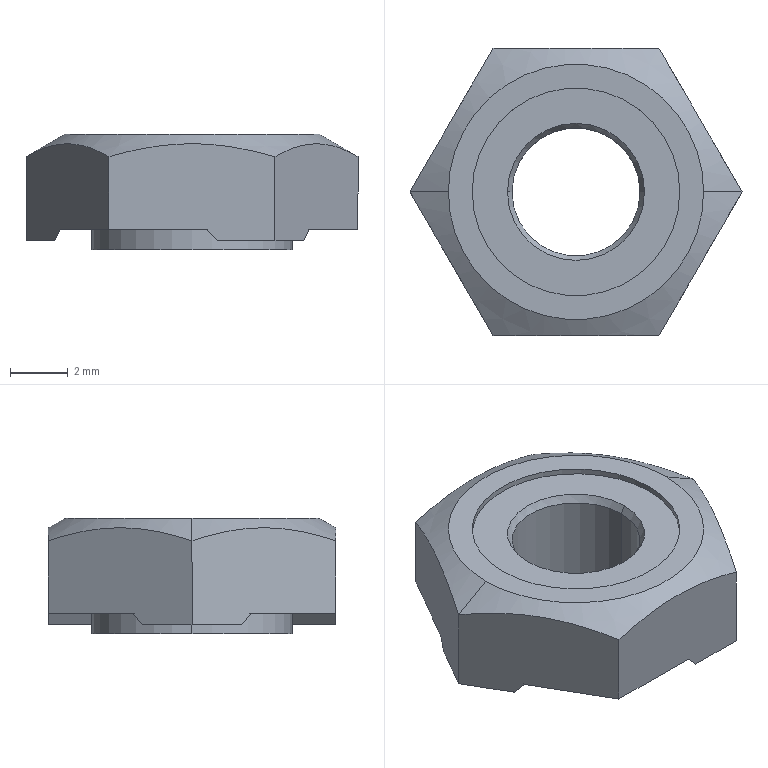Part | SolidWorks | features Cut 2, RevCut 2, Boss 1, Chamfer 1, CirPattern 1, Draft 1, Extrusion 1, LPattern 1, RefAxis 1 | 1 solid | 28 faces | box 11.547 x 10 x 4 mm | volume 240.353 mm3 | plane 16 | cone 6 | cylinder 6 | commonest cylinder face diameters 4.459 x2 6.96 x2 7.22 x2
STEP:
#1=CARTESIAN_POINT('',(-2.229,0.,-0.4667));
#2=VERTEX_POINT('',#1);
#3=CARTESIAN_POINT('',(2.229,0.,-0.4667));
#4=VERTEX_POINT('',#3);
#5=CARTESIAN_POINT('',(0.,0.,-0.4667));
#6=DIRECTION('',(0.,0.,1.));
#7=DIRECTION('',(-1.,0.,0.));
#8=AXIS2_PLACEMENT_3D('',#5,#6,#7);
#9=CIRCLE('',#8,2.229);
#10=EDGE_CURVE('',#2,#4,#9,.T.);
#11=ORIENTED_EDGE('',*,*,#10,.F.);
#12=CARTESIAN_POINT('',(-2.383,0.,-0.2));
#13=VERTEX_POINT('',#12);
#14=CARTESIAN_POINT('',(-2.383,0.,-0.2));
#15=DIRECTION('',(-0.5,0.,0.866));
#16=VECTOR('',#15,1000.);
#17=LINE('',#14,#16);
#18=EDGE_CURVE('',#2,#13,#17,.T.);
#19=ORIENTED_EDGE('',*,*,#18,.T.);
#20=CARTESIAN_POINT('',(2.383,0.,-0.2));
#21=VERTEX_POINT('',#20);
#22=CARTESIAN_POINT('',(0.,0.,-0.2));
#23=DIRECTION('',(0.,0.,-1.));
#24=DIRECTION('',(-1.,0.,0.));
#25=AXIS2_PLACEMENT_3D('',#22,#23,#24);
#26=CIRCLE('',#25,2.383);
#27=EDGE_CURVE('',#21,#13,#26,.T.);
#28=ORIENTED_EDGE('',*,*,#27,.F.);
#29=CARTESIAN_POINT('',(2.383,0.,-0.2));
#30=DIRECTION('',(0.5,0.,0.866));
#31=VECTOR('',#30,1000.);
#32=LINE('',#29,#31);
#33=EDGE_CURVE('',#4,#21,#32,.T.);
#34=ORIENTED_EDGE('',*,*,#33,.F.);
#35=EDGE_LOOP('',(#11,#19,#28,#34));
#36=FACE_OUTER_BOUND('',#35,.T.);
#37=CARTESIAN_POINT('',(0.,0.,-0.2));
#38=DIRECTION('',(0.,0.,1.));
#39=DIRECTION('',(1.,0.,0.));
#40=AXIS2_PLACEMENT_3D('',#37,#38,#39);
#41=CONICAL_SURFACE('',#40,2.383,0.5236);
#42=ADVANCED_FACE('',(#36),#41,.F.);
#43=CARTESIAN_POINT('',(2.229,0.,-3.846));
#44=VERTEX_POINT('',#43);
#45=CARTESIAN_POINT('',(-2.229,0.,-3.846));
#46=VERTEX_POINT('',#45);
#47=CARTESIAN_POINT('',(0.,0.,-3.846));
#48=DIRECTION('',(0.,0.,-1.));
#49=DIRECTION('',(1.,0.,0.));
#50=AXIS2_PLACEMENT_3D('',#47,#48,#49);
#51=CIRCLE('',#50,2.229);
#52=EDGE_CURVE('',#44,#46,#51,.T.);
#53=ORIENTED_EDGE('',*,*,#52,.F.);
#54=CARTESIAN_POINT('',(2.496,0.,-4.));
#55=VERTEX_POINT('',#54);
#56=CARTESIAN_POINT('',(2.229,0.,-3.846));
#57=DIRECTION('',(0.866,0.,-0.5));
#58=VECTOR('',#57,1000.);
#59=LINE('',#56,#58);
#60=EDGE_CURVE('',#44,#55,#59,.T.);
#61=ORIENTED_EDGE('',*,*,#60,.T.);
#62=CARTESIAN_POINT('',(-2.496,0.,-4.));
#63=VERTEX_POINT('',#62);
#64=CARTESIAN_POINT('',(0.,0.,-4.));
#65=DIRECTION('',(0.,0.,1.));
#66=DIRECTION('',(1.,0.,0.));
#67=AXIS2_PLACEMENT_3D('',#64,#65,#66);
#68=CIRCLE('',#67,2.496);
#69=EDGE_CURVE('',#63,#55,#68,.T.);
#70=ORIENTED_EDGE('',*,*,#69,.F.);
#71=CARTESIAN_POINT('',(-2.229,0.,-3.846));
#72=DIRECTION('',(-0.866,0.,-0.5));
#73=VECTOR('',#72,1000.);
#74=LINE('',#71,#73);
#75=EDGE_CURVE('',#46,#63,#74,.T.);
#76=ORIENTED_EDGE('',*,*,#75,.F.);
#77=EDGE_LOOP('',(#53,#61,#70,#76));
#78=FACE_OUTER_BOUND('',#77,.T.);
#79=CARTESIAN_POINT('',(0.,0.,-3.846));
#80=DIRECTION('',(0.,0.,-1.));
#81=DIRECTION('',(-1.,0.,0.));
#82=AXIS2_PLACEMENT_3D('',#79,#80,#81);
#83=CONICAL_SURFACE('',#82,2.229,1.047);
#84=ADVANCED_FACE('',(#78),#83,.F.);
#85=ORIENTED_EDGE('',*,*,#10,.T.);
#86=CARTESIAN_POINT('',(2.229,0.,0.));
#87=DIRECTION('',(0.,0.,-1.));
#88=VECTOR('',#87,1000.);
#89=LINE('',#86,#88);
#90=EDGE_CURVE('',#4,#44,#89,.T.);
#91=ORIENTED_EDGE('',*,*,#90,.T.);
#92=ORIENTED_EDGE('',*,*,#52,.T.);
#93=CARTESIAN_POINT('',(-2.229,0.,0.));
#94=DIRECTION('',(0.,0.,-1.));
#95=VECTOR('',#94,1000.);
#96=LINE('',#93,#95);
#97=EDGE_CURVE('',#2,#46,#96,.T.);
#98=ORIENTED_EDGE('',*,*,#97,.F.);
#99=EDGE_LOOP('',(#85,#91,#92,#98));
#100=FACE_OUTER_BOUND('',#99,.T.);
#101=CARTESIAN_POINT('',(0.,0.,0.));
#102=DIRECTION('',(0.,0.,-1.));
#103=DIRECTION('',(-1.,0.,0.));
#104=AXIS2_PLACEMENT_3D('',#101,#102,#103);
#105=CYLINDRICAL_SURFACE('',#104,2.229);
#106=ADVANCED_FACE('',(#100),#105,.F.);
#107=CARTESIAN_POINT('',(-3.48,0.,-3.3));
#108=VERTEX_POINT('',#107);
#109=CARTESIAN_POINT('',(3.48,0.,-3.3));
#110=VERTEX_POINT('',#109);
#111=CARTESIAN_POINT('',(0.,0.,-3.3));
#112=DIRECTION('',(0.,0.,-1.));
#113=DIRECTION('',(-1.,0.,0.));
#114=AXIS2_PLACEMENT_3D('',#111,#112,#113);
#115=CIRCLE('',#114,3.48);
#116=EDGE_CURVE('',#108,#110,#115,.T.);
#117=ORIENTED_EDGE('',*,*,#116,.T.);
#118=CARTESIAN_POINT('',(3.48,0.,-4.));
#119=VERTEX_POINT('',#118);
#120=CARTESIAN_POINT('',(3.48,0.,-3.3));
#121=DIRECTION('',(0.,0.,-1.));
#122=VECTOR('',#121,1000.);
#123=LINE('',#120,#122);
#124=EDGE_CURVE('',#110,#119,#123,.T.);
#125=ORIENTED_EDGE('',*,*,#124,.T.);
#126=CARTESIAN_POINT('',(-3.48,0.,-4.));
#127=VERTEX_POINT('',#126);
#128=CARTESIAN_POINT('',(0.,0.,-4.));
#129=DIRECTION('',(0.,0.,-1.));
#130=DIRECTION('',(-1.,0.,0.));
#131=AXIS2_PLACEMENT_3D('',#128,#129,#130);
#132=CIRCLE('',#131,3.48);
#133=EDGE_CURVE('',#127,#119,#132,.T.);
#134=ORIENTED_EDGE('',*,*,#133,.F.);
#135=CARTESIAN_POINT('',(-3.48,0.,-3.3));
#136=DIRECTION('',(0.,0.,-1.));
#137=VECTOR('',#136,1000.);
#138=LINE('',#135,#137);
#139=EDGE_CURVE('',#108,#127,#138,.T.);
#140=ORIENTED_EDGE('',*,*,#139,.F.);
#141=EDGE_LOOP('',(#117,#125,#134,#140));
#142=FACE_OUTER_BOUND('',#141,.T.);
#143=CARTESIAN_POINT('',(0.,0.,-3.3));
#144=DIRECTION('',(0.,0.,-1.));
#145=DIRECTION('',(-1.,0.,0.));
#146=AXIS2_PLACEMENT_3D('',#143,#144,#145);
#147=CYLINDRICAL_SURFACE('',#146,3.48);
#148=ADVANCED_FACE('',(#142),#147,.T.);
#149=CARTESIAN_POINT('',(3.61,0.,0.));
#150=VERTEX_POINT('',#149);
#151=CARTESIAN_POINT('',(-3.61,0.,0.));
#152=VERTEX_POINT('',#151);
#153=CARTESIAN_POINT('',(0.,0.,0.));
#154=DIRECTION('',(0.,0.,-1.));
#155=DIRECTION('',(-1.,0.,0.));
#156=AXIS2_PLACEMENT_3D('',#153,#154,#155);
#157=CIRCLE('',#156,3.61);
#158=EDGE_CURVE('',#150,#152,#157,.T.);
#159=ORIENTED_EDGE('',*,*,#158,.F.);
#160=CARTESIAN_POINT('',(3.61,0.,-0.2));
#161=VERTEX_POINT('',#160);
#162=CARTESIAN_POINT('',(3.61,0.,-9.902));
#163=DIRECTION('',(0.,0.,-1.));
#164=VECTOR('',#163,1000.);
#165=LINE('',#162,#164);
#166=EDGE_CURVE('',#150,#161,#165,.T.);
#167=ORIENTED_EDGE('',*,*,#166,.T.);
#168=CARTESIAN_POINT('',(-3.61,0.,-0.2));
#169=VERTEX_POINT('',#168);
#170=CARTESIAN_POINT('',(0.,0.,-0.2));
#171=DIRECTION('',(0.,0.,-1.));
#172=DIRECTION('',(-1.,0.,0.));
#173=AXIS2_PLACEMENT_3D('',#170,#171,#172);
#174=CIRCLE('',#173,3.61);
#175=EDGE_CURVE('',#161,#169,#174,.T.);
#176=ORIENTED_EDGE('',*,*,#175,.T.);
#177=CARTESIAN_POINT('',(-3.61,0.,-9.902));
#178=DIRECTION('',(0.,0.,-1.));
#179=VECTOR('',#178,1000.);
#180=LINE('',#177,#179);
#181=EDGE_CURVE('',#152,#169,#180,.T.);
#182=ORIENTED_EDGE('',*,*,#181,.F.);
#183=EDGE_LOOP('',(#159,#167,#176,#182));
#184=FACE_OUTER_BOUND('',#183,.T.);
#185=CARTESIAN_POINT('',(0.,0.,-9.902));
#186=DIRECTION('',(0.,0.,-1.));
#187=DIRECTION('',(-1.,0.,0.));
#188=AXIS2_PLACEMENT_3D('',#185,#186,#187);
#189=CYLINDRICAL_SURFACE('',#188,3.61);
#190=ADVANCED_FACE('',(#184),#189,.F.);
#191=CARTESIAN_POINT('',(-4.44,0.,0.));
#192=VERTEX_POINT('',#191);
#193=CARTESIAN_POINT('',(4.44,0.,0.));
#194=VERTEX_POINT('',#193);
#195=CARTESIAN_POINT('',(0.,0.,0.));
#196=DIRECTION('',(0.,0.,-1.));
#197=DIRECTION('',(-1.,0.,0.));
#198=AXIS2_PLACEMENT_3D('',#195,#196,#197);
#199=CIRCLE('',#198,4.44);
#200=EDGE_CURVE('',#192,#194,#199,.T.);
#201=ORIENTED_EDGE('',*,*,#200,.T.);
#202=CARTESIAN_POINT('',(5.774,0.,-0.7699));
#203=VERTEX_POINT('',#202);
#204=CARTESIAN_POINT('',(4.44,0.,0.));
#205=DIRECTION('',(0.866,0.,-0.5));
#206=VECTOR('',#205,1000.);
#207=LINE('',#204,#206);
#208=EDGE_CURVE('',#194,#203,#207,.T.);
#209=ORIENTED_EDGE('',*,*,#208,.T.);
#210=CARTESIAN_POINT('',(2.887,5.,-0.7699));
#211=VERTEX_POINT('',#210);
#212=CARTESIAN_POINT('',(5.774,0.,-0.7699));
#213=CARTESIAN_POINT('',(5.302,0.8164,-0.4978));
#214=CARTESIAN_POINT('',(4.824,1.645,-0.3239));
#215=CARTESIAN_POINT('',(4.21,2.708,-0.3232));
#216=CARTESIAN_POINT('',(4.087,2.921,-0.3336));
#217=CARTESIAN_POINT('',(3.843,3.344,-0.3743));
#218=CARTESIAN_POINT('',(3.722,3.554,-0.4045));
#219=CARTESIAN_POINT('',(3.361,4.179,-0.5212));
#220=CARTESIAN_POINT('',(3.123,4.591,-0.6337));
#221=CARTESIAN_POINT('',(2.887,5.,-0.7699));
#222=B_SPLINE_CURVE_WITH_KNOTS('',3,(#212,#213,#214,#215,#216,#217,#218,#219,#220,#221),.UNSPECIFIED.,.F.,.F.,(4,2,2,2,4),(0.000000238,0.002916,0.003645,0.004373,0.005831),.UNSPECIFIED.);
#223=EDGE_CURVE('',#203,#211,#222,.T.);
#224=ORIENTED_EDGE('',*,*,#223,.T.);
#225=CARTESIAN_POINT('',(-2.887,5.,-0.7699));
#226=VERTEX_POINT('',#225);
#227=CARTESIAN_POINT('',(2.887,5.,-0.7699));
#228=CARTESIAN_POINT('',(2.42,5.,-0.6352));
#229=CARTESIAN_POINT('',(1.947,5.,-0.523));
#230=CARTESIAN_POINT('',(0.9831,5.,-0.3664));
#231=CARTESIAN_POINT('',(0.4886,5.,-0.3234));
#232=CARTESIAN_POINT('',(-0.487,5.,-0.3233));
#233=CARTESIAN_POINT('',(-0.9718,5.,-0.3652));
#234=CARTESIAN_POINT('',(-1.936,5.,-0.5206));
#235=CARTESIAN_POINT('',(-2.417,5.,-0.6344));
#236=CARTESIAN_POINT('',(-2.887,5.,-0.7699));
#237=B_SPLINE_CURVE_WITH_KNOTS('',3,(#227,#228,#229,#230,#231,#232,#233,#234,#235,#236),.UNSPECIFIED.,.F.,.F.,(4,2,2,2,4),(0.01286,0.01432,0.01578,0.01724,0.01871),.UNSPECIFIED.);
#238=EDGE_CURVE('',#211,#226,#237,.T.);
#239=ORIENTED_EDGE('',*,*,#238,.T.);
#240=CARTESIAN_POINT('',(-5.774,0.,-0.7699));
#241=VERTEX_POINT('',#240);
#242=CARTESIAN_POINT('',(-2.887,5.,-0.7699));
#243=CARTESIAN_POINT('',(-3.358,4.184,-0.4978));
#244=CARTESIAN_POINT('',(-3.837,3.355,-0.3239));
#245=CARTESIAN_POINT('',(-4.45,2.292,-0.3232));
#246=CARTESIAN_POINT('',(-4.573,2.079,-0.3336));
#247=CARTESIAN_POINT('',(-4.817,1.656,-0.3743));
#248=CARTESIAN_POINT('',(-4.938,1.446,-0.4045));
#249=CARTESIAN_POINT('',(-5.3,0.8208,-0.5212));
#250=CARTESIAN_POINT('',(-5.538,0.4087,-0.6337));
#251=CARTESIAN_POINT('',(-5.774,0.,-0.7699));
#252=B_SPLINE_CURVE_WITH_KNOTS('',3,(#242,#243,#244,#245,#246,#247,#248,#249,#250,#251),.UNSPECIFIED.,.F.,.F.,(4,2,2,2,4),(0.000000238,0.002916,0.003645,0.004373,0.005831),.UNSPECIFIED.);
#253=EDGE_CURVE('',#226,#241,#252,.T.);
#254=ORIENTED_EDGE('',*,*,#253,.T.);
#255=CARTESIAN_POINT('',(-4.44,0.,0.));
#256=DIRECTION('',(-0.866,0.,-0.5));
#257=VECTOR('',#256,1000.);
#258=LINE('',#255,#257);
#259=EDGE_CURVE('',#192,#241,#258,.T.);
#260=ORIENTED_EDGE('',*,*,#259,.F.);
#261=EDGE_LOOP('',(#201,#209,#224,#239,#254,#260));
#262=FACE_OUTER_BOUND('',#261,.T.);
#263=CARTESIAN_POINT('',(0.,0.,0.));
#264=DIRECTION('',(0.,0.,-1.));
#265=DIRECTION('',(-1.,0.,0.));
#266=AXIS2_PLACEMENT_3D('',#263,#264,#265);
#267=CONICAL_SURFACE('',#266,4.44,1.047);
#268=ADVANCED_FACE('',(#262),#267,.T.);
#269=ORIENTED_EDGE('',*,*,#116,.F.);
#270=CARTESIAN_POINT('',(0.,0.,-3.3));
#271=DIRECTION('',(0.,0.,-1.));
#272=DIRECTION('',(-1.,0.,0.));
#273=AXIS2_PLACEMENT_3D('',#270,#271,#272);
#274=CIRCLE('',#273,3.48);
#275=EDGE_CURVE('',#110,#108,#274,.T.);
#276=ORIENTED_EDGE('',*,*,#275,.F.);
#277=EDGE_LOOP('',(#269,#276));
#278=FACE_BOUND('',#277,.T.);
#279=CARTESIAN_POINT('',(-4.587,-2.055,-3.3));
#280=VERTEX_POINT('',#279);
#281=CARTESIAN_POINT('',(-2.887,-5.,-3.3));
#282=VERTEX_POINT('',#281);
#283=CARTESIAN_POINT('',(-5.774,0.,-3.3));
#284=DIRECTION('',(0.5,-0.866,0.));
#285=VECTOR('',#284,1000.);
#286=LINE('',#283,#285);
#287=EDGE_CURVE('',#280,#282,#286,.T.);
#288=ORIENTED_EDGE('',*,*,#287,.F.);
#289=CARTESIAN_POINT('',(-4.587,2.055,-3.3));
#290=VERTEX_POINT('',#289);
#291=CARTESIAN_POINT('',(-4.587,1.732,-3.3));
#292=DIRECTION('',(0.,-1.,0.));
#293=VECTOR('',#292,1000.);
#294=LINE('',#291,#293);
#295=EDGE_CURVE('',#290,#280,#294,.T.);
#296=ORIENTED_EDGE('',*,*,#295,.F.);
#297=CARTESIAN_POINT('',(-2.887,5.,-3.3));
#298=VERTEX_POINT('',#297);
#299=CARTESIAN_POINT('',(-2.887,5.,-3.3));
#300=DIRECTION('',(-0.5,-0.866,0.));
#301=VECTOR('',#300,1000.);
#302=LINE('',#299,#301);
#303=EDGE_CURVE('',#298,#290,#302,.T.);
#304=ORIENTED_EDGE('',*,*,#303,.F.);
#305=CARTESIAN_POINT('',(0.5137,5.,-3.3));
#306=VERTEX_POINT('',#305);
#307=CARTESIAN_POINT('',(2.887,5.,-3.3));
#308=DIRECTION('',(-1.,0.,0.));
#309=VECTOR('',#308,1000.);
#310=LINE('',#307,#309);
#311=EDGE_CURVE('',#306,#298,#310,.T.);
#312=ORIENTED_EDGE('',*,*,#311,.F.);
#313=CARTESIAN_POINT('',(4.073,2.945,-3.3));
#314=VERTEX_POINT('',#313);
#315=CARTESIAN_POINT('',(3.793,3.106,-3.3));
#316=DIRECTION('',(-0.866,0.5,0.));
#317=VECTOR('',#316,1000.);
#318=LINE('',#315,#317);
#319=EDGE_CURVE('',#314,#306,#318,.T.);
#320=ORIENTED_EDGE('',*,*,#319,.F.);
#321=CARTESIAN_POINT('',(5.774,0.,-3.3));
#322=VERTEX_POINT('',#321);
#323=CARTESIAN_POINT('',(5.774,0.,-3.3));
#324=DIRECTION('',(-0.5,0.866,0.));
#325=VECTOR('',#324,1000.);
#326=LINE('',#323,#325);
#327=EDGE_CURVE('',#322,#314,#326,.T.);
#328=ORIENTED_EDGE('',*,*,#327,.F.);
#329=CARTESIAN_POINT('',(4.073,-2.945,-3.3));
#330=VERTEX_POINT('',#329);
#331=CARTESIAN_POINT('',(2.887,-5.,-3.3));
#332=DIRECTION('',(0.5,0.866,0.));
#333=VECTOR('',#332,1000.);
#334=LINE('',#331,#333);
#335=EDGE_CURVE('',#330,#322,#334,.T.);
#336=ORIENTED_EDGE('',*,*,#335,.F.);
#337=CARTESIAN_POINT('',(0.5137,-5.,-3.3));
#338=VERTEX_POINT('',#337);
#339=CARTESIAN_POINT('',(0.7935,-4.838,-3.3));
#340=DIRECTION('',(0.866,0.5,0.));
#341=VECTOR('',#340,1000.);
#342=LINE('',#339,#341);
#343=EDGE_CURVE('',#338,#330,#342,.T.);
#344=ORIENTED_EDGE('',*,*,#343,.F.);
#345=CARTESIAN_POINT('',(-2.887,-5.,-3.3));
#346=DIRECTION('',(1.,0.,0.));
#347=VECTOR('',#346,1000.);
#348=LINE('',#345,#347);
#349=EDGE_CURVE('',#282,#338,#348,.T.);
#350=ORIENTED_EDGE('',*,*,#349,.F.);
#351=EDGE_LOOP('',(#288,#296,#304,#312,#320,#328,#336,#344,#350));
#352=FACE_OUTER_BOUND('',#351,.T.);
#353=CARTESIAN_POINT('',(0.,0.,-3.3));
#354=DIRECTION('',(0.,0.,-1.));
#355=DIRECTION('',(-1.,0.,0.));
#356=AXIS2_PLACEMENT_3D('',#353,#354,#355);
#357=PLANE('',#356);
#358=ADVANCED_FACE('',(#278,#352),#357,.T.);
#359=CARTESIAN_POINT('',(-2.887,-5.,-0.7699));
#360=VERTEX_POINT('',#359);
#361=CARTESIAN_POINT('',(-2.887,-5.,-4.));
#362=DIRECTION('',(0.,0.,1.));
#363=VECTOR('',#362,1000.);
#364=LINE('',#361,#363);
#365=EDGE_CURVE('',#282,#360,#364,.T.);
#366=ORIENTED_EDGE('',*,*,#365,.F.);
#367=ORIENTED_EDGE('',*,*,#349,.T.);
#368=CARTESIAN_POINT('',(0.8868,-5.,-3.7));
#369=VERTEX_POINT('',#368);
#370=CARTESIAN_POINT('',(-0.719,-5.,-1.978));
#371=DIRECTION('',(-0.682,0.,0.7313));
#372=VECTOR('',#371,1000.);
#373=LINE('',#370,#372);
#374=EDGE_CURVE('',#369,#338,#373,.T.);
#375=ORIENTED_EDGE('',*,*,#374,.F.);
#376=CARTESIAN_POINT('',(2.887,-5.,-3.7));
#377=VERTEX_POINT('',#376);
#378=CARTESIAN_POINT('',(2.887,-5.,-3.7));
#379=DIRECTION('',(-1.,0.,0.));
#380=VECTOR('',#379,1000.);
#381=LINE('',#378,#380);
#382=EDGE_CURVE('',#377,#369,#381,.T.);
#383=ORIENTED_EDGE('',*,*,#382,.F.);
#384=CARTESIAN_POINT('',(2.887,-5.,-0.7699));
#385=VERTEX_POINT('',#384);
#386=CARTESIAN_POINT('',(2.887,-5.,-4.));
#387=DIRECTION('',(0.,0.,1.));
#388=VECTOR('',#387,1000.);
#389=LINE('',#386,#388);
#390=EDGE_CURVE('',#377,#385,#389,.T.);
#391=ORIENTED_EDGE('',*,*,#390,.T.);
#392=CARTESIAN_POINT('',(-2.887,-5.,-0.7699));
#393=CARTESIAN_POINT('',(-2.417,-5.,-0.6344));
#394=CARTESIAN_POINT('',(-1.936,-5.,-0.5206));
#395=CARTESIAN_POINT('',(-0.9718,-5.,-0.3652));
#396=CARTESIAN_POINT('',(-0.487,-5.,-0.3233));
#397=CARTESIAN_POINT('',(0.4886,-5.,-0.3234));
#398=CARTESIAN_POINT('',(0.9831,-5.,-0.3664));
#399=CARTESIAN_POINT('',(1.947,-5.,-0.523));
#400=CARTESIAN_POINT('',(2.42,-5.,-0.6352));
#401=CARTESIAN_POINT('',(2.887,-5.,-0.7699));
#402=B_SPLINE_CURVE_WITH_KNOTS('',3,(#392,#393,#394,#395,#396,#397,#398,#399,#400,#401),.UNSPECIFIED.,.F.,.F.,(4,2,2,2,4),(0.005101,0.006561,0.008021,0.009482,0.01094),.UNSPECIFIED.);
#403=EDGE_CURVE('',#360,#385,#402,.T.);
#404=ORIENTED_EDGE('',*,*,#403,.F.);
#405=EDGE_LOOP('',(#366,#367,#375,#383,#391,#404));
#406=FACE_OUTER_BOUND('',#405,.T.);
#407=CARTESIAN_POINT('',(-2.887,-5.,-4.));
#408=DIRECTION('',(0.,-1.,0.));
#409=DIRECTION('',(0.,0.,-1.));
#410=AXIS2_PLACEMENT_3D('',#407,#408,#409);
#411=PLANE('',#410);
#412=ADVANCED_FACE('',(#406),#411,.T.);
#413=CARTESIAN_POINT('',(-5.774,0.,-3.7));
#414=VERTEX_POINT('',#413);
#415=CARTESIAN_POINT('',(-5.774,0.,-4.));
#416=DIRECTION('',(0.,0.,1.));
#417=VECTOR('',#416,1000.);
#418=LINE('',#415,#417);
#419=EDGE_CURVE('',#414,#241,#418,.T.);
#420=ORIENTED_EDGE('',*,*,#419,.F.);
#421=CARTESIAN_POINT('',(-4.774,-1.732,-3.7));
#422=VERTEX_POINT('',#421);
#423=CARTESIAN_POINT('',(-4.774,-1.732,-3.7));
#424=DIRECTION('',(-0.5,0.866,0.));
#425=VECTOR('',#424,1000.);
#426=LINE('',#423,#425);
#427=EDGE_CURVE('',#422,#414,#426,.T.);
#428=ORIENTED_EDGE('',*,*,#427,.F.);
#429=CARTESIAN_POINT('',(-5.471,-0.5235,-5.196));
#430=DIRECTION('',(0.341,-0.5907,0.7313));
#431=VECTOR('',#430,1000.);
#432=LINE('',#429,#431);
#433=EDGE_CURVE('',#422,#280,#432,.T.);
#434=ORIENTED_EDGE('',*,*,#433,.T.);
#435=ORIENTED_EDGE('',*,*,#287,.T.);
#436=ORIENTED_EDGE('',*,*,#365,.T.);
#437=CARTESIAN_POINT('',(-5.774,0.,-0.7699));
#438=CARTESIAN_POINT('',(-5.302,-0.8164,-0.4978));
#439=CARTESIAN_POINT('',(-4.824,-1.645,-0.3239));
#440=CARTESIAN_POINT('',(-4.21,-2.708,-0.3232));
#441=CARTESIAN_POINT('',(-4.087,-2.921,-0.3336));
#442=CARTESIAN_POINT('',(-3.843,-3.344,-0.3743));
#443=CARTESIAN_POINT('',(-3.722,-3.554,-0.4045));
#444=CARTESIAN_POINT('',(-3.361,-4.179,-0.5212));
#445=CARTESIAN_POINT('',(-3.123,-4.591,-0.6337));
#446=CARTESIAN_POINT('',(-2.887,-5.,-0.7699));
#447=B_SPLINE_CURVE_WITH_KNOTS('',3,(#437,#438,#439,#440,#441,#442,#443,#444,#445,#446),.UNSPECIFIED.,.F.,.F.,(4,2,2,2,4),(0.000000238,0.002916,0.003645,0.004373,0.005831),.UNSPECIFIED.);
#448=EDGE_CURVE('',#241,#360,#447,.T.);
#449=ORIENTED_EDGE('',*,*,#448,.F.);
#450=EDGE_LOOP('',(#420,#428,#434,#435,#436,#449));
#451=FACE_OUTER_BOUND('',#450,.T.);
#452=CARTESIAN_POINT('',(-5.774,0.,-4.));
#453=DIRECTION('',(-0.866,-0.5,0.));
#454=DIRECTION('',(0.5,-0.866,0.));
#455=AXIS2_PLACEMENT_3D('',#452,#453,#454);
#456=PLANE('',#455);
#457=ADVANCED_FACE('',(#451),#456,.T.);
#458=CARTESIAN_POINT('',(-2.887,5.,-4.));
#459=DIRECTION('',(0.,0.,1.));
#460=VECTOR('',#459,1000.);
#461=LINE('',#458,#460);
#462=EDGE_CURVE('',#298,#226,#461,.T.);
#463=ORIENTED_EDGE('',*,*,#462,.F.);
#464=ORIENTED_EDGE('',*,*,#303,.T.);
#465=CARTESIAN_POINT('',(-4.774,1.732,-3.7));
#466=VERTEX_POINT('',#465);
#467=CARTESIAN_POINT('',(-3.971,3.123,-1.978));
#468=DIRECTION('',(0.341,0.5907,0.7313));
#469=VECTOR('',#468,1000.);
#470=LINE('',#467,#469);
#471=EDGE_CURVE('',#466,#290,#470,.T.);
#472=ORIENTED_EDGE('',*,*,#471,.F.);
#473=CARTESIAN_POINT('',(-5.774,0.,-3.7));
#474=DIRECTION('',(0.5,0.866,0.));
#475=VECTOR('',#474,1000.);
#476=LINE('',#473,#475);
#477=EDGE_CURVE('',#414,#466,#476,.T.);
#478=ORIENTED_EDGE('',*,*,#477,.F.);
#479=ORIENTED_EDGE('',*,*,#419,.T.);
#480=ORIENTED_EDGE('',*,*,#253,.F.);
#481=EDGE_LOOP('',(#463,#464,#472,#478,#479,#480));
#482=FACE_OUTER_BOUND('',#481,.T.);
#483=CARTESIAN_POINT('',(-2.887,5.,-4.));
#484=DIRECTION('',(-0.866,0.5,0.));
#485=DIRECTION('',(-0.5,-0.866,0.));
#486=AXIS2_PLACEMENT_3D('',#483,#484,#485);
#487=PLANE('',#486);
#488=ADVANCED_FACE('',(#482),#487,.T.);
#489=CARTESIAN_POINT('',(2.887,5.,-3.7));
#490=VERTEX_POINT('',#489);
#491=CARTESIAN_POINT('',(2.887,5.,-4.));
#492=DIRECTION('',(0.,0.,1.));
#493=VECTOR('',#492,1000.);
#494=LINE('',#491,#493);
#495=EDGE_CURVE('',#490,#211,#494,.T.);
#496=ORIENTED_EDGE('',*,*,#495,.F.);
#497=CARTESIAN_POINT('',(0.8868,5.,-3.7));
#498=VERTEX_POINT('',#497);
#499=CARTESIAN_POINT('',(0.8868,5.,-3.7));
#500=DIRECTION('',(1.,0.,0.));
#501=VECTOR('',#500,1000.);
#502=LINE('',#499,#501);
#503=EDGE_CURVE('',#498,#490,#502,.T.);
#504=ORIENTED_EDGE('',*,*,#503,.F.);
#505=CARTESIAN_POINT('',(2.282,5.,-5.196));
#506=DIRECTION('',(-0.682,0.,0.7313));
#507=VECTOR('',#506,1000.);
#508=LINE('',#505,#507);
#509=EDGE_CURVE('',#498,#306,#508,.T.);
#510=ORIENTED_EDGE('',*,*,#509,.T.);
#511=ORIENTED_EDGE('',*,*,#311,.T.);
#512=ORIENTED_EDGE('',*,*,#462,.T.);
#513=ORIENTED_EDGE('',*,*,#238,.F.);
#514=EDGE_LOOP('',(#496,#504,#510,#511,#512,#513));
#515=FACE_OUTER_BOUND('',#514,.T.);
#516=CARTESIAN_POINT('',(2.887,5.,-4.));
#517=DIRECTION('',(0.,1.,0.));
#518=DIRECTION('',(0.,0.,1.));
#519=AXIS2_PLACEMENT_3D('',#516,#517,#518);
#520=PLANE('',#519);
#521=ADVANCED_FACE('',(#515),#520,.T.);
#522=CARTESIAN_POINT('',(5.774,0.,-4.));
#523=DIRECTION('',(0.,0.,1.));
#524=VECTOR('',#523,1000.);
#525=LINE('',#522,#524);
#526=EDGE_CURVE('',#322,#203,#525,.T.);
#527=ORIENTED_EDGE('',*,*,#526,.F.);
#528=ORIENTED_EDGE('',*,*,#327,.T.);
#529=CARTESIAN_POINT('',(3.887,3.268,-3.7));
#530=VERTEX_POINT('',#529);
#531=CARTESIAN_POINT('',(4.69,1.877,-1.978));
#532=DIRECTION('',(0.341,-0.5907,0.7313));
#533=VECTOR('',#532,1000.);
#534=LINE('',#531,#533);
#535=EDGE_CURVE('',#530,#314,#534,.T.);
#536=ORIENTED_EDGE('',*,*,#535,.F.);
#537=CARTESIAN_POINT('',(2.887,5.,-3.7));
#538=DIRECTION('',(0.5,-0.866,0.));
#539=VECTOR('',#538,1000.);
#540=LINE('',#537,#539);
#541=EDGE_CURVE('',#490,#530,#540,.T.);
#542=ORIENTED_EDGE('',*,*,#541,.F.);
#543=ORIENTED_EDGE('',*,*,#495,.T.);
#544=ORIENTED_EDGE('',*,*,#223,.F.);
#545=EDGE_LOOP('',(#527,#528,#536,#542,#543,#544));
#546=FACE_OUTER_BOUND('',#545,.T.);
#547=CARTESIAN_POINT('',(5.774,0.,-4.));
#548=DIRECTION('',(0.866,0.5,0.));
#549=DIRECTION('',(-0.5,0.866,0.));
#550=AXIS2_PLACEMENT_3D('',#547,#548,#549);
#551=PLANE('',#550);
#552=ADVANCED_FACE('',(#546),#551,.T.);
#553=ORIENTED_EDGE('',*,*,#390,.F.);
#554=CARTESIAN_POINT('',(3.887,-3.268,-3.7));
#555=VERTEX_POINT('',#554);
#556=CARTESIAN_POINT('',(3.887,-3.268,-3.7));
#557=DIRECTION('',(-0.5,-0.866,0.));
#558=VECTOR('',#557,1000.);
#559=LINE('',#556,#558);
#560=EDGE_CURVE('',#555,#377,#559,.T.);
#561=ORIENTED_EDGE('',*,*,#560,.F.);
#562=CARTESIAN_POINT('',(3.189,-4.477,-5.196));
#563=DIRECTION('',(0.341,0.5907,0.7313));
#564=VECTOR('',#563,1000.);
#565=LINE('',#562,#564);
#566=EDGE_CURVE('',#555,#330,#565,.T.);
#567=ORIENTED_EDGE('',*,*,#566,.T.);
#568=ORIENTED_EDGE('',*,*,#335,.T.);
#569=ORIENTED_EDGE('',*,*,#526,.T.);
#570=CARTESIAN_POINT('',(2.887,-5.,-0.7699));
#571=CARTESIAN_POINT('',(3.358,-4.184,-0.4978));
#572=CARTESIAN_POINT('',(3.837,-3.355,-0.3239));
#573=CARTESIAN_POINT('',(4.45,-2.292,-0.3232));
#574=CARTESIAN_POINT('',(4.573,-2.079,-0.3336));
#575=CARTESIAN_POINT('',(4.817,-1.656,-0.3743));
#576=CARTESIAN_POINT('',(4.938,-1.446,-0.4045));
#577=CARTESIAN_POINT('',(5.3,-0.8208,-0.5212));
#578=CARTESIAN_POINT('',(5.538,-0.4087,-0.6337));
#579=CARTESIAN_POINT('',(5.774,0.,-0.7699));
#580=B_SPLINE_CURVE_WITH_KNOTS('',3,(#570,#571,#572,#573,#574,#575,#576,#577,#578,#579),.UNSPECIFIED.,.F.,.F.,(4,2,2,2,4),(0.000000238,0.002916,0.003645,0.004373,0.005831),.UNSPECIFIED.);
#581=EDGE_CURVE('',#385,#203,#580,.T.);
#582=ORIENTED_EDGE('',*,*,#581,.F.);
#583=EDGE_LOOP('',(#553,#561,#567,#568,#569,#582));
#584=FACE_OUTER_BOUND('',#583,.T.);
#585=CARTESIAN_POINT('',(2.887,-5.,-4.));
#586=DIRECTION('',(0.866,-0.5,0.));
#587=DIRECTION('',(0.5,0.866,0.));
#588=AXIS2_PLACEMENT_3D('',#585,#586,#587);
#589=PLANE('',#588);
#590=ADVANCED_FACE('',(#584),#589,.T.);
#591=ORIENTED_EDGE('',*,*,#208,.F.);
#592=CARTESIAN_POINT('',(0.,0.,0.));
#593=DIRECTION('',(0.,0.,-1.));
#594=DIRECTION('',(-1.,0.,0.));
#595=AXIS2_PLACEMENT_3D('',#592,#593,#594);
#596=CIRCLE('',#595,4.44);
#597=EDGE_CURVE('',#194,#192,#596,.T.);
#598=ORIENTED_EDGE('',*,*,#597,.T.);
#599=ORIENTED_EDGE('',*,*,#259,.T.);
#600=ORIENTED_EDGE('',*,*,#448,.T.);
#601=ORIENTED_EDGE('',*,*,#403,.T.);
#602=ORIENTED_EDGE('',*,*,#581,.T.);
#603=EDGE_LOOP('',(#591,#598,#599,#600,#601,#602));
#604=FACE_OUTER_BOUND('',#603,.T.);
#605=CARTESIAN_POINT('',(0.,0.,0.));
#606=DIRECTION('',(0.,0.,-1.));
#607=DIRECTION('',(-1.,0.,0.));
#608=AXIS2_PLACEMENT_3D('',#605,#606,#607);
#609=CONICAL_SURFACE('',#608,4.44,1.047);
#610=ADVANCED_FACE('',(#604),#609,.T.);
#611=CARTESIAN_POINT('',(0.,0.,0.));
#612=DIRECTION('',(0.,0.,-1.));
#613=DIRECTION('',(-1.,0.,0.));
#614=AXIS2_PLACEMENT_3D('',#611,#612,#613);
#615=CIRCLE('',#614,3.61);
#616=EDGE_CURVE('',#152,#150,#615,.T.);
#617=ORIENTED_EDGE('',*,*,#616,.T.);
#618=ORIENTED_EDGE('',*,*,#158,.T.);
#619=EDGE_LOOP('',(#617,#618));
#620=FACE_BOUND('',#619,.T.);
#621=ORIENTED_EDGE('',*,*,#200,.F.);
#622=ORIENTED_EDGE('',*,*,#597,.F.);
#623=EDGE_LOOP('',(#621,#622));
#624=FACE_OUTER_BOUND('',#623,.T.);
#625=CARTESIAN_POINT('',(2.887,-5.,0.));
#626=DIRECTION('',(0.,0.,1.));
#627=DIRECTION('',(1.,0.,0.));
#628=AXIS2_PLACEMENT_3D('',#625,#626,#627);
#629=PLANE('',#628);
#630=ADVANCED_FACE('',(#620,#624),#629,.T.);
#631=ORIENTED_EDGE('',*,*,#166,.F.);
#632=ORIENTED_EDGE('',*,*,#616,.F.);
#633=ORIENTED_EDGE('',*,*,#181,.T.);
#634=CARTESIAN_POINT('',(0.,0.,-0.2));
#635=DIRECTION('',(0.,0.,-1.));
#636=DIRECTION('',(-1.,0.,0.));
#637=AXIS2_PLACEMENT_3D('',#634,#635,#636);
#638=CIRCLE('',#637,3.61);
#639=EDGE_CURVE('',#169,#161,#638,.T.);
#640=ORIENTED_EDGE('',*,*,#639,.T.);
#641=EDGE_LOOP('',(#631,#632,#633,#640));
#642=FACE_OUTER_BOUND('',#641,.T.);
#643=CARTESIAN_POINT('',(0.,0.,-9.902));
#644=DIRECTION('',(0.,0.,-1.));
#645=DIRECTION('',(-1.,0.,0.));
#646=AXIS2_PLACEMENT_3D('',#643,#644,#645);
#647=CYLINDRICAL_SURFACE('',#646,3.61);
#648=ADVANCED_FACE('',(#642),#647,.F.);
#649=ORIENTED_EDGE('',*,*,#27,.T.);
#650=CARTESIAN_POINT('',(0.,0.,-0.2));
#651=DIRECTION('',(0.,0.,-1.));
#652=DIRECTION('',(-1.,0.,0.));
#653=AXIS2_PLACEMENT_3D('',#650,#651,#652);
#654=CIRCLE('',#653,2.383);
#655=EDGE_CURVE('',#13,#21,#654,.T.);
#656=ORIENTED_EDGE('',*,*,#655,.T.);
#657=EDGE_LOOP('',(#649,#656));
#658=FACE_BOUND('',#657,.T.);
#659=ORIENTED_EDGE('',*,*,#639,.F.);
#660=ORIENTED_EDGE('',*,*,#175,.F.);
#661=EDGE_LOOP('',(#659,#660));
#662=FACE_OUTER_BOUND('',#661,.T.);
#663=CARTESIAN_POINT('',(0.,0.,-0.2));
#664=DIRECTION('',(0.,0.,-1.));
#665=DIRECTION('',(-1.,0.,0.));
#666=AXIS2_PLACEMENT_3D('',#663,#664,#665);
#667=PLANE('',#666);
#668=ADVANCED_FACE('',(#658,#662),#667,.F.);
#669=ORIENTED_EDGE('',*,*,#124,.F.);
#670=ORIENTED_EDGE('',*,*,#275,.T.);
#671=ORIENTED_EDGE('',*,*,#139,.T.);
#672=CARTESIAN_POINT('',(0.,0.,-4.));
#673=DIRECTION('',(0.,0.,-1.));
#674=DIRECTION('',(-1.,0.,0.));
#675=AXIS2_PLACEMENT_3D('',#672,#673,#674);
#676=CIRCLE('',#675,3.48);
#677=EDGE_CURVE('',#119,#127,#676,.T.);
#678=ORIENTED_EDGE('',*,*,#677,.F.);
#679=EDGE_LOOP('',(#669,#670,#671,#678));
#680=FACE_OUTER_BOUND('',#679,.T.);
#681=CARTESIAN_POINT('',(0.,0.,-3.3));
#682=DIRECTION('',(0.,0.,-1.));
#683=DIRECTION('',(-1.,0.,0.));
#684=AXIS2_PLACEMENT_3D('',#681,#682,#683);
#685=CYLINDRICAL_SURFACE('',#684,3.48);
#686=ADVANCED_FACE('',(#680),#685,.T.);
#687=ORIENTED_EDGE('',*,*,#69,.T.);
#688=CARTESIAN_POINT('',(0.,0.,-4.));
#689=DIRECTION('',(0.,0.,1.));
#690=DIRECTION('',(1.,0.,0.));
#691=AXIS2_PLACEMENT_3D('',#688,#689,#690);
#692=CIRCLE('',#691,2.496);
#693=EDGE_CURVE('',#55,#63,#692,.T.);
#694=ORIENTED_EDGE('',*,*,#693,.T.);
#695=EDGE_LOOP('',(#687,#694));
#696=FACE_BOUND('',#695,.T.);
#697=ORIENTED_EDGE('',*,*,#133,.T.);
#698=ORIENTED_EDGE('',*,*,#677,.T.);
#699=EDGE_LOOP('',(#697,#698));
#700=FACE_OUTER_BOUND('',#699,.T.);
#701=CARTESIAN_POINT('',(2.887,-5.,-4.));
#702=DIRECTION('',(0.,0.,1.));
#703=DIRECTION('',(1.,0.,0.));
#704=AXIS2_PLACEMENT_3D('',#701,#702,#703);
#705=PLANE('',#704);
#706=ADVANCED_FACE('',(#696,#700),#705,.F.);
#707=ORIENTED_EDGE('',*,*,#343,.T.);
#708=ORIENTED_EDGE('',*,*,#566,.F.);
#709=CARTESIAN_POINT('',(0.8868,-5.,-3.7));
#710=DIRECTION('',(0.866,0.5,0.));
#711=VECTOR('',#710,1000.);
#712=LINE('',#709,#711);
#713=EDGE_CURVE('',#369,#555,#712,.T.);
#714=ORIENTED_EDGE('',*,*,#713,.F.);
#715=ORIENTED_EDGE('',*,*,#374,.T.);
#716=EDGE_LOOP('',(#707,#708,#714,#715));
#717=FACE_OUTER_BOUND('',#716,.T.);
#718=CARTESIAN_POINT('',(0.8868,-5.,-3.7));
#719=DIRECTION('',(-0.4532,0.7849,-0.4226));
#720=DIRECTION('',(-0.866,-0.5,0.));
#721=AXIS2_PLACEMENT_3D('',#718,#719,#720);
#722=PLANE('',#721);
#723=ADVANCED_FACE('',(#717),#722,.T.);
#724=ORIENTED_EDGE('',*,*,#560,.T.);
#725=ORIENTED_EDGE('',*,*,#382,.T.);
#726=ORIENTED_EDGE('',*,*,#713,.T.);
#727=EDGE_LOOP('',(#724,#725,#726));
#728=FACE_OUTER_BOUND('',#727,.T.);
#729=CARTESIAN_POINT('',(2.887,-5.,-3.7));
#730=DIRECTION('',(0.,0.,-1.));
#731=DIRECTION('',(-1.,0.,0.));
#732=AXIS2_PLACEMENT_3D('',#729,#730,#731);
#733=PLANE('',#732);
#734=ADVANCED_FACE('',(#728),#733,.T.);
#735=ORIENTED_EDGE('',*,*,#319,.T.);
#736=ORIENTED_EDGE('',*,*,#509,.F.);
#737=CARTESIAN_POINT('',(3.887,3.268,-3.7));
#738=DIRECTION('',(-0.866,0.5,0.));
#739=VECTOR('',#738,1000.);
#740=LINE('',#737,#739);
#741=EDGE_CURVE('',#530,#498,#740,.T.);
#742=ORIENTED_EDGE('',*,*,#741,.F.);
#743=ORIENTED_EDGE('',*,*,#535,.T.);
#744=EDGE_LOOP('',(#735,#736,#742,#743));
#745=FACE_OUTER_BOUND('',#744,.T.);
#746=CARTESIAN_POINT('',(3.887,3.268,-3.7));
#747=DIRECTION('',(-0.4532,-0.7849,-0.4226));
#748=DIRECTION('',(0.866,-0.5,0.));
#749=AXIS2_PLACEMENT_3D('',#746,#747,#748);
#750=PLANE('',#749);
#751=ADVANCED_FACE('',(#745),#750,.T.);
#752=ORIENTED_EDGE('',*,*,#503,.T.);
#753=ORIENTED_EDGE('',*,*,#541,.T.);
#754=ORIENTED_EDGE('',*,*,#741,.T.);
#755=EDGE_LOOP('',(#752,#753,#754));
#756=FACE_OUTER_BOUND('',#755,.T.);
#757=CARTESIAN_POINT('',(2.887,5.,-3.7));
#758=DIRECTION('',(0.,0.,-1.));
#759=DIRECTION('',(0.5,-0.866,0.));
#760=AXIS2_PLACEMENT_3D('',#757,#758,#759);
#761=PLANE('',#760);
#762=ADVANCED_FACE('',(#756),#761,.T.);
#763=ORIENTED_EDGE('',*,*,#295,.T.);
#764=ORIENTED_EDGE('',*,*,#433,.F.);
#765=CARTESIAN_POINT('',(-4.774,1.732,-3.7));
#766=DIRECTION('',(0.,-1.,0.));
#767=VECTOR('',#766,1000.);
#768=LINE('',#765,#767);
#769=EDGE_CURVE('',#466,#422,#768,.T.);
#770=ORIENTED_EDGE('',*,*,#769,.F.);
#771=ORIENTED_EDGE('',*,*,#471,.T.);
#772=EDGE_LOOP('',(#763,#764,#770,#771));
#773=FACE_OUTER_BOUND('',#772,.T.);
#774=CARTESIAN_POINT('',(-4.774,1.732,-3.7));
#775=DIRECTION('',(0.9063,0.,-0.4226));
#776=DIRECTION('',(-0.4226,0.,-0.9063));
#777=AXIS2_PLACEMENT_3D('',#774,#775,#776);
#778=PLANE('',#777);
#779=ADVANCED_FACE('',(#773),#778,.T.);
#780=ORIENTED_EDGE('',*,*,#427,.T.);
#781=ORIENTED_EDGE('',*,*,#477,.T.);
#782=ORIENTED_EDGE('',*,*,#769,.T.);
#783=EDGE_LOOP('',(#780,#781,#782));
#784=FACE_OUTER_BOUND('',#783,.T.);
#785=CARTESIAN_POINT('',(-5.774,0.,-3.7));
#786=DIRECTION('',(0.,0.,-1.));
#787=DIRECTION('',(0.5,0.866,0.));
#788=AXIS2_PLACEMENT_3D('',#785,#786,#787);
#789=PLANE('',#788);
#790=ADVANCED_FACE('',(#784),#789,.T.);
#791=ORIENTED_EDGE('',*,*,#90,.F.);
#792=CARTESIAN_POINT('',(0.,0.,-0.4667));
#793=DIRECTION('',(0.,0.,1.));
#794=DIRECTION('',(-1.,0.,0.));
#795=AXIS2_PLACEMENT_3D('',#792,#793,#794);
#796=CIRCLE('',#795,2.229);
#797=EDGE_CURVE('',#4,#2,#796,.T.);
#798=ORIENTED_EDGE('',*,*,#797,.T.);
#799=ORIENTED_EDGE('',*,*,#97,.T.);
#800=CARTESIAN_POINT('',(0.,0.,-3.846));
#801=DIRECTION('',(0.,0.,-1.));
#802=DIRECTION('',(1.,0.,0.));
#803=AXIS2_PLACEMENT_3D('',#800,#801,#802);
#804=CIRCLE('',#803,2.229);
#805=EDGE_CURVE('',#46,#44,#804,.T.);
#806=ORIENTED_EDGE('',*,*,#805,.T.);
#807=EDGE_LOOP('',(#791,#798,#799,#806));
#808=FACE_OUTER_BOUND('',#807,.T.);
#809=CARTESIAN_POINT('',(0.,0.,0.));
#810=DIRECTION('',(0.,0.,-1.));
#811=DIRECTION('',(-1.,0.,0.));
#812=AXIS2_PLACEMENT_3D('',#809,#810,#811);
#813=CYLINDRICAL_SURFACE('',#812,2.229);
#814=ADVANCED_FACE('',(#808),#813,.F.);
#815=ORIENTED_EDGE('',*,*,#60,.F.);
#816=ORIENTED_EDGE('',*,*,#805,.F.);
#817=ORIENTED_EDGE('',*,*,#75,.T.);
#818=ORIENTED_EDGE('',*,*,#693,.F.);
#819=EDGE_LOOP('',(#815,#816,#817,#818));
#820=FACE_OUTER_BOUND('',#819,.T.);
#821=CARTESIAN_POINT('',(0.,0.,-3.846));
#822=DIRECTION('',(0.,0.,-1.));
#823=DIRECTION('',(-1.,0.,0.));
#824=AXIS2_PLACEMENT_3D('',#821,#822,#823);
#825=CONICAL_SURFACE('',#824,2.229,1.047);
#826=ADVANCED_FACE('',(#820),#825,.F.);
#827=ORIENTED_EDGE('',*,*,#18,.F.);
#828=ORIENTED_EDGE('',*,*,#797,.F.);
#829=ORIENTED_EDGE('',*,*,#33,.T.);
#830=ORIENTED_EDGE('',*,*,#655,.F.);
#831=EDGE_LOOP('',(#827,#828,#829,#830));
#832=FACE_OUTER_BOUND('',#831,.T.);
#833=CARTESIAN_POINT('',(0.,0.,-0.2));
#834=DIRECTION('',(0.,0.,1.));
#835=DIRECTION('',(1.,0.,0.));
#836=AXIS2_PLACEMENT_3D('',#833,#834,#835);
#837=CONICAL_SURFACE('',#836,2.383,0.5236);
#838=ADVANCED_FACE('',(#832),#837,.F.);
#839=CLOSED_SHELL('',(#42,#84,#106,#148,#190,#268,#358,#412,#457,#488,#521,#552,#590,#610,#630,#648,#668,#686,#706,#723,#734,#751,#762,#779,#790,#814,#826,#838));
#840=MANIFOLD_SOLID_BREP('',#839);
#841=CARTESIAN_POINT('',(0.,0.,0.));
#842=DIRECTION('',(0.,0.,1.));
#843=DIRECTION('',(1.,0.,0.));
#844=AXIS2_PLACEMENT_3D('',#841,#842,#843);
#845=(LENGTH_UNIT()NAMED_UNIT(*)SI_UNIT(.MILLI.,.METRE.));
#846=UNCERTAINTY_MEASURE_WITH_UNIT(LENGTH_MEASURE(0.00001),#845,'','');
#847=(NAMED_UNIT(*)PLANE_ANGLE_UNIT()SI_UNIT($,.RADIAN.));
#848=(NAMED_UNIT(*)SI_UNIT($,.STERADIAN.)SOLID_ANGLE_UNIT());
#849=(GEOMETRIC_REPRESENTATION_CONTEXT(3)GLOBAL_UNCERTAINTY_ASSIGNED_CONTEXT((#846))GLOBAL_UNIT_ASSIGNED_CONTEXT((#845,#847,#848))REPRESENTATION_CONTEXT('',''));
#850=ADVANCED_BREP_SHAPE_REPRESENTATION('',(#840,#844),#849);